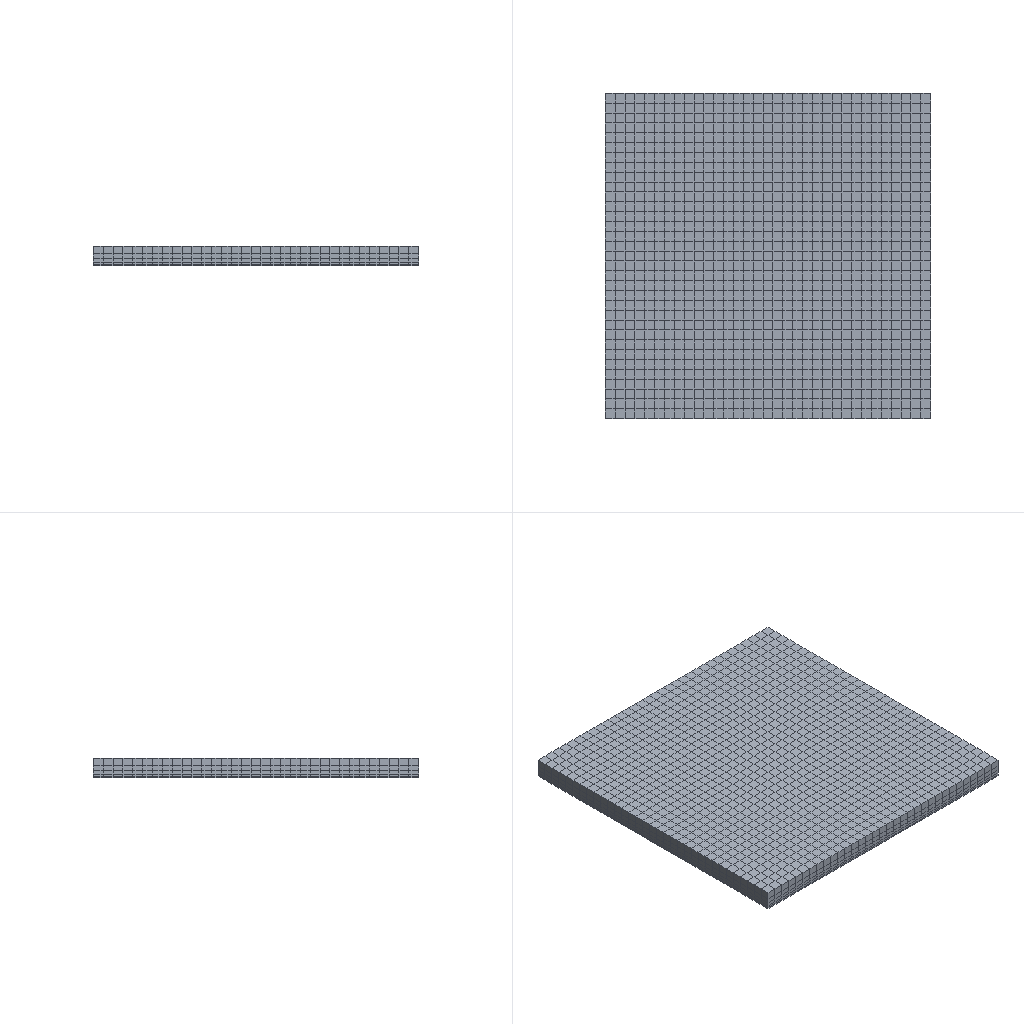Simulation study | abaqus
Set-up summary:
category,name,step,type,value,unit,region
solver,abaqus
solver,version,,,Abaqus/Explicit 2020
units,not stated in the deck,,not stated
analysis,deck,,transient,transient
load_step,Step-1,Step-1,transient,nlgeom=True
load_step,Step-2,Step-2,transient,nlgeom=True
load_step,Step-3,Step-3,transient,nlgeom=True
contact,interactions,,,general=0 pairs=1 ties=0
load_step,requested,,,3
mesh,nodes,,,7583
mesh,elements,,,6099
element_type,R3D3,,rigid,20
element_type,R3D4,,rigid,634
element_type,C3D8R,,solid,5445
load,load commands in deck,,count,5
bc,support commands in deck,,count,12
material,MATERIAL-1,,in results
check,setup vs results,,match,"per instance, exact: element labels, types and connectivity; labels of the nodes the elements use; coordinates of those nodes at SINGLE_PRECISION in 2 of 2 instance(s)"
Abaqus input file, long lists of numbers shortened:
*Heading
** Job name: Job-1 Model name: Model-1
** Generated by: Abaqus/CAE 2020
*Preprint, echo=NO, model=NO, history=NO, contact=NO
**
** PARTS
**
*Part, name=tool-5
*Node
      1,   1035.955,  -100.285,   790.01
      2,   1035.955,   15.548,   866.844
** (644 more lines like these left out)
*Element, type=R3D4
 1,  1,  5, 54,  4
 2,  5,  6, 53, 54
** (632 more lines like these left out)
*Element, type=R3D3
53, 184, 349, 186
54, 235, 334, 225
** (18 more lines like these left out)
*Node
    647,   1035.955,  -42.368,   828.427
*Nset, nset=tool-5-RefPt_, internal
647,
*Elset, elset=tool-5, generate
   1,  654,    1
*End Part
**
*Part, name=work
*Node
      1,           0.,        -500.,          30.
      2,           0.,   -484.848,          30.
** (6934 more lines like these left out)
*Element, type=C3D8R
   1,  205,  206,  240,  239,    1,    2,   36,   35
   2,  206,  207,  241,  240,    2,    3,   37,   36
** (5443 more lines like these left out)
*Nset, nset=Set-1, generate
    1,  6936,     1
*Elset, elset=Set-1, generate
    1,  5445,     1
** Section: Section-1
*Solid Section, elset=Set-1, material=Material-1
,
*End Part
**
**
** ASSEMBLY
**
*Assembly, name=Assembly
**
*Instance, name=tool-5-1, part=tool-5
 -908.427,  -242.368, -1038.955
 -908.427,  -242.368, -1038.955, -907.72,  -242.368, -1038.248,         180.
*End Instance
**
*Instance, name=work-1, part=work
*End Instance
**
*Nset, nset=Set-2, instance=tool-5-1
 647,
*Nset, nset=Set-3, instance=work-1
    1,    2,    3,    4,    5,    6,    7,    8,    9,   10,   11,   12,   13,   14,   15,   16
   17,   18,   19,   20,   21,   22,   23,   24,   25,   26,   27,   28,   29,   30,   31,   32
** (71 more lines like these left out)
*Elset, elset=Set-3, instance=work-1
    1,    2,    3,    4,    5,    6,    7,    8,    9,   10,   11,   12,   13,   14,   15,   16
   17,   18,   19,   20,   21,   22,   23,   24,   25,   26,   27,   28,   29,   30,   31,   32
** (67 more lines like these left out)
*Nset, nset=s_Set-1, instance=work-1, generate
    1,  6936,     1
*Elset, elset=s_Set-1, instance=work-1, generate
    1,  5445,     1
*Elset, elset=_m_Surf-1_SPOS, internal, instance=tool-5-1, generate
   1,  654,    1
*Surface, type=ELEMENT, name=m_Surf-1
_m_Surf-1_SPOS, SPOS
*Surface, type=NODE, name=s_Set-1_CNS_, internal
s_Set-1, 1.
*Rigid Body, ref node=tool-5-1.tool-5-RefPt_, elset=tool-5-1.tool-5
*End Assembly
**
** MATERIALS
**
*Material, name=Material-1
*Damage Initiation, criterion=JOHNSON COOK
 -0.09,  0.25,  -0.5, 0.014,  3.87, 1650.,   25.,    1.
*Damage Evolution, type=DISPLACEMENT
 0.001,
*Density
 4.4e-09,
*Elastic
108000., 0.33
*Plastic, hardening=JOHNSON COOK
860., 683., 0.47,   1.,1650.,  25.
*Rate Dependent, type=JOHNSON COOK
 0.035,1.
**
** INTERACTION PROPERTIES
**
*Surface Interaction, name=IntProp-1
*Friction
 0.1,
*Surface Behavior, pressure-overclosure=HARD
** ----------------------------------------------------------------
**
** STEP: Step-1
**
*Step, name=Step-1, nlgeom=YES
*Dynamic, Explicit
, 0.1
*Bulk Viscosity
0.06, 1.2
** Mass Scaling: Semi-Automatic
**               Whole Model
*Fixed Mass Scaling, factor=500.
**
** BOUNDARY CONDITIONS
**
** Name: BC-2 Type: 对称/反对称/完全固定
*Boundary
Set-3, ENCASTRE
** Name: [REDACTED] : Velocity/Angular velocity
*Boundary, type=VELOCITY
Set-2, 1, 1, 6000.
Set-2, 2, 2
Set-2, 3, 3
Set-2, 4, 4
Set-2, 5, 5
Set-2, 6, 6, 628.
**
** INTERACTIONS
**
** Interaction: Int-1
*Contact Pair, interaction=IntProp-1, mechanical constraint=KINEMATIC, cpset=Int-1
m_Surf-1, s_Set-1_CNS_
**
** OUTPUT REQUESTS
**
*Restart, write, number interval=1, time marks=NO
**
** FIELD OUTPUT: F-Output-1
**
*Output, field, number interval=30
*Node Output
A, CF, RF, RM, RT, U, V
*Element Output, directions=YES
E, EVF, HP, LE, MISES, MISESMAX, MISESONLY, NE, NFORC, P, PE, PEEQ, PEEQMAX, PEEQT, PEEQVAVG, PEMAG
PEVAVG, PRESSONLY, S, SDEG, SEQUT, SF, SSAVG, STATUS, SVAVG, TSHR, YIELDPOT
*Contact Output
CDISP, CFORCE, CSDMG, CSTRESS, FSLIP, FSLIPR
**
** HISTORY OUTPUT: H-Output-1
**
*Output, history, variable=PRESELECT
*End Step
** ----------------------------------------------------------------
**
** STEP: Step-2
**
*Step, name=Step-2, nlgeom=YES
*Dynamic, Explicit
, 0.1
*Bulk Viscosity
0.06, 1.2
** Mass Scaling: Semi-Automatic
**               Whole Model
*Fixed Mass Scaling, factor=500.
**
** BOUNDARY CONDITIONS
**
** Name: [REDACTED] : Velocity/Angular velocity
*Boundary, type=VELOCITY
Set-2, 1, 1
Set-2, 2, 2, -750.
**
** OUTPUT REQUESTS
**
*Restart, write, number interval=1, time marks=NO
**
** FIELD OUTPUT: F-Output-1
**
*Output, field, number interval=5
*Node Output
A, CF, RF, RM, RT, U, V
*Element Output, directions=YES
E, EVF, HP, LE, MISES, MISESMAX, MISESONLY, NE, NFORC, P, PE, PEEQ, PEEQMAX, PEEQT, PEEQVAVG, PEMAG
PEVAVG, PRESSONLY, S, SDEG, SEQUT, SF, SSAVG, STATUS, SVAVG, TSHR, YIELDPOT
*Contact Output
CDISP, CFORCE, CSDMG, CSTRESS, FSLIP, FSLIPR
**
** HISTORY OUTPUT: H-Output-1
**
*Output, history, variable=PRESELECT
*End Step
** ----------------------------------------------------------------
**
** STEP: Step-3
**
*Step, name=Step-3, nlgeom=YES
*Dynamic, Explicit
, 0.1
*Bulk Viscosity
0.06, 1.2
** Mass Scaling: Semi-Automatic
**               Whole Model
*Fixed Mass Scaling, factor=500.
**
** BOUNDARY CONDITIONS
**
** Name: [REDACTED] : Velocity/Angular velocity
*Boundary, type=VELOCITY
Set-2, 1, 1, -6000.
Set-2, 2, 2
Set-2, 6, 6, 628.
**
** OUTPUT REQUESTS
**
*Restart, write, number interval=1, time marks=NO
**
** FIELD OUTPUT: F-Output-1
**
*Output, field, number interval=30
*Node Output
A, CF, RF, RM, RT, U, V
*Element Output, directions=YES
E, EVF, HP, LE, MISES, MISESMAX, MISESONLY, NE, NFORC, P, PE, PEEQ, PEEQMAX, PEEQT, PEEQVAVG, PEMAG
PEVAVG, PRESSONLY, S, SDEG, SEQUT, SF, SSAVG, STATUS, SVAVG, TSHR, YIELDPOT
*Contact Output
CDISP, CFORCE, CSDMG, CSTRESS, FSLIP, FSLIPR
**
** HISTORY OUTPUT: H-Output-1
**
*Output, history, variable=PRESELECT
*End Step
Results summary:
result,step,Step-1,completed,increments=11764 time=0.1/0.1
result,step,Step-2,completed,increments=11765 time=0.1/0.1
result,step,Step-3,completed,increments=11765 time=0.1/0.1
result,analysis,,,transient
result,last_loadstep,,,3
result,analysis steps,,count,3
result,primary field,,,U
result,reaction total,,FX,-154358.671,model units
result,reaction total,,FY,1378932.993,model units
result,reaction total,,FZ,20048.187,model units